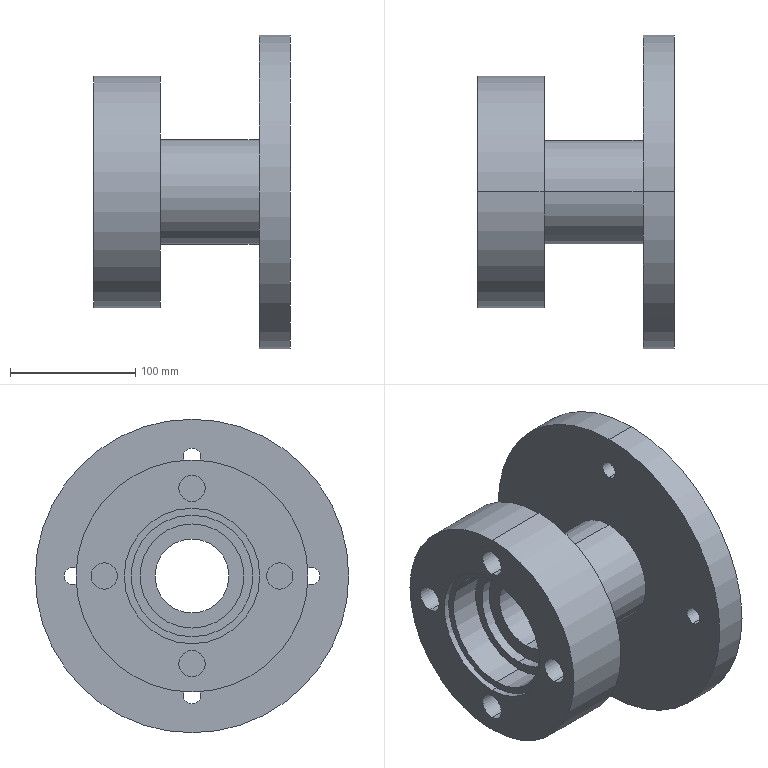Part | STEP file | Coupling | 2 solids | 43 faces | box 157 x 250 x 250 mm | volume 2335528 mm3 | cylinder 34 | plane 9 | commonest cylinder face diameters 14 x8 21 x8 83 x6 59 x2 96 x2 97 x2